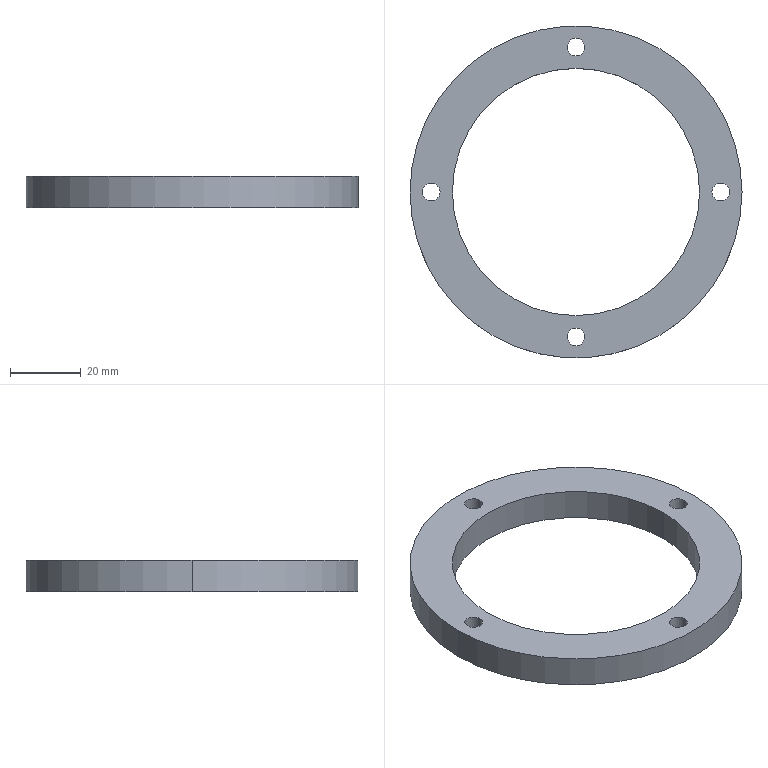Part | SolidWorks | features BaseBody 1 | 1 solid | 14 faces | box 94 x 94 x 9 mm | volume 27115 mm3 | cylinder 12 | plane 2 | commonest cylinder face diameters 5 x8 70 x2 94 x2
STEP:
#1=CARTESIAN_POINT('',(35.,0.,9.));
#2=VERTEX_POINT('',#1);
#3=CARTESIAN_POINT('',(-35.,0.,9.));
#4=VERTEX_POINT('',#3);
#5=CARTESIAN_POINT('',(0.,0.,9.));
#6=DIRECTION('',(0.,0.,-1.));
#7=DIRECTION('',(-1.,0.,0.));
#8=AXIS2_PLACEMENT_3D('',#5,#6,#7);
#9=CIRCLE('',#8,35.);
#10=EDGE_CURVE('',#2,#4,#9,.T.);
#11=ORIENTED_EDGE('',*,*,#10,.F.);
#12=CARTESIAN_POINT('',(35.,0.,0.));
#13=VERTEX_POINT('',#12);
#14=CARTESIAN_POINT('',(35.,0.,9.));
#15=DIRECTION('',(0.,0.,-1.));
#16=VECTOR('',#15,1000.);
#17=LINE('',#14,#16);
#18=EDGE_CURVE('',#2,#13,#17,.T.);
#19=ORIENTED_EDGE('',*,*,#18,.T.);
#20=CARTESIAN_POINT('',(-35.,0.,0.));
#21=VERTEX_POINT('',#20);
#22=CARTESIAN_POINT('',(0.,0.,0.));
#23=DIRECTION('',(0.,0.,1.));
#24=DIRECTION('',(-1.,0.,0.));
#25=AXIS2_PLACEMENT_3D('',#22,#23,#24);
#26=CIRCLE('',#25,35.);
#27=EDGE_CURVE('',#21,#13,#26,.T.);
#28=ORIENTED_EDGE('',*,*,#27,.F.);
#29=CARTESIAN_POINT('',(-35.,0.,9.));
#30=DIRECTION('',(0.,0.,-1.));
#31=VECTOR('',#30,1000.);
#32=LINE('',#29,#31);
#33=EDGE_CURVE('',#4,#21,#32,.T.);
#34=ORIENTED_EDGE('',*,*,#33,.F.);
#35=EDGE_LOOP('',(#11,#19,#28,#34));
#36=FACE_OUTER_BOUND('',#35,.T.);
#37=CARTESIAN_POINT('',(0.,0.,9.));
#38=DIRECTION('',(0.,0.,-1.));
#39=DIRECTION('',(-1.,0.,0.));
#40=AXIS2_PLACEMENT_3D('',#37,#38,#39);
#41=CYLINDRICAL_SURFACE('',#40,35.);
#42=ADVANCED_FACE('',(#36),#41,.F.);
#43=CARTESIAN_POINT('',(47.,0.,9.));
#44=VERTEX_POINT('',#43);
#45=CARTESIAN_POINT('',(-47.,0.,9.));
#46=VERTEX_POINT('',#45);
#47=CARTESIAN_POINT('',(0.,0.,9.));
#48=DIRECTION('',(0.,0.,1.));
#49=DIRECTION('',(-1.,0.,0.));
#50=AXIS2_PLACEMENT_3D('',#47,#48,#49);
#51=CIRCLE('',#50,47.);
#52=EDGE_CURVE('',#44,#46,#51,.T.);
#53=ORIENTED_EDGE('',*,*,#52,.F.);
#54=CARTESIAN_POINT('',(47.,0.,0.));
#55=VERTEX_POINT('',#54);
#56=CARTESIAN_POINT('',(47.,0.,9.));
#57=DIRECTION('',(0.,0.,-1.));
#58=VECTOR('',#57,1000.);
#59=LINE('',#56,#58);
#60=EDGE_CURVE('',#44,#55,#59,.T.);
#61=ORIENTED_EDGE('',*,*,#60,.T.);
#62=CARTESIAN_POINT('',(-47.,0.,0.));
#63=VERTEX_POINT('',#62);
#64=CARTESIAN_POINT('',(0.,0.,0.));
#65=DIRECTION('',(0.,0.,1.));
#66=DIRECTION('',(-1.,0.,0.));
#67=AXIS2_PLACEMENT_3D('',#64,#65,#66);
#68=CIRCLE('',#67,47.);
#69=EDGE_CURVE('',#55,#63,#68,.T.);
#70=ORIENTED_EDGE('',*,*,#69,.T.);
#71=CARTESIAN_POINT('',(-47.,0.,9.));
#72=DIRECTION('',(0.,0.,-1.));
#73=VECTOR('',#72,1000.);
#74=LINE('',#71,#73);
#75=EDGE_CURVE('',#46,#63,#74,.T.);
#76=ORIENTED_EDGE('',*,*,#75,.F.);
#77=EDGE_LOOP('',(#53,#61,#70,#76));
#78=FACE_OUTER_BOUND('',#77,.T.);
#79=CARTESIAN_POINT('',(0.,0.,9.));
#80=DIRECTION('',(0.,0.,-1.));
#81=DIRECTION('',(-1.,0.,0.));
#82=AXIS2_PLACEMENT_3D('',#79,#80,#81);
#83=CYLINDRICAL_SURFACE('',#82,47.);
#84=ADVANCED_FACE('',(#78),#83,.T.);
#85=CARTESIAN_POINT('',(-43.5,0.,0.));
#86=VERTEX_POINT('',#85);
#87=CARTESIAN_POINT('',(-38.5,0.,0.));
#88=VERTEX_POINT('',#87);
#89=CARTESIAN_POINT('',(-41.,0.,0.));
#90=DIRECTION('',(0.,0.,1.));
#91=DIRECTION('',(1.,0.,0.));
#92=AXIS2_PLACEMENT_3D('',#89,#90,#91);
#93=CIRCLE('',#92,2.5);
#94=EDGE_CURVE('',#86,#88,#93,.T.);
#95=ORIENTED_EDGE('',*,*,#94,.F.);
#96=CARTESIAN_POINT('',(-43.5,0.,9.));
#97=VERTEX_POINT('',#96);
#98=CARTESIAN_POINT('',(-43.5,0.,-34.));
#99=DIRECTION('',(0.,0.,1.));
#100=VECTOR('',#99,1000.);
#101=LINE('',#98,#100);
#102=EDGE_CURVE('',#86,#97,#101,.T.);
#103=ORIENTED_EDGE('',*,*,#102,.T.);
#104=CARTESIAN_POINT('',(-38.5,0.,9.));
#105=VERTEX_POINT('',#104);
#106=CARTESIAN_POINT('',(-41.,0.,9.));
#107=DIRECTION('',(0.,0.,-1.));
#108=DIRECTION('',(1.,0.,0.));
#109=AXIS2_PLACEMENT_3D('',#106,#107,#108);
#110=CIRCLE('',#109,2.5);
#111=EDGE_CURVE('',#105,#97,#110,.T.);
#112=ORIENTED_EDGE('',*,*,#111,.F.);
#113=CARTESIAN_POINT('',(-38.5,0.,-34.));
#114=DIRECTION('',(0.,0.,1.));
#115=VECTOR('',#114,1000.);
#116=LINE('',#113,#115);
#117=EDGE_CURVE('',#88,#105,#116,.T.);
#118=ORIENTED_EDGE('',*,*,#117,.F.);
#119=EDGE_LOOP('',(#95,#103,#112,#118));
#120=FACE_OUTER_BOUND('',#119,.T.);
#121=CARTESIAN_POINT('',(-41.,0.,-34.));
#122=DIRECTION('',(0.,0.,1.));
#123=DIRECTION('',(1.,0.,0.));
#124=AXIS2_PLACEMENT_3D('',#121,#122,#123);
#125=CYLINDRICAL_SURFACE('',#124,2.5);
#126=ADVANCED_FACE('',(#120),#125,.F.);
#127=CARTESIAN_POINT('',(-2.5,-41.,0.));
#128=VERTEX_POINT('',#127);
#129=CARTESIAN_POINT('',(2.5,-41.,0.));
#130=VERTEX_POINT('',#129);
#131=CARTESIAN_POINT('',(0.,-41.,0.));
#132=DIRECTION('',(0.,0.,1.));
#133=DIRECTION('',(1.,0.,0.));
#134=AXIS2_PLACEMENT_3D('',#131,#132,#133);
#135=CIRCLE('',#134,2.5);
#136=EDGE_CURVE('',#128,#130,#135,.T.);
#137=ORIENTED_EDGE('',*,*,#136,.F.);
#138=CARTESIAN_POINT('',(-2.5,-41.,9.));
#139=VERTEX_POINT('',#138);
#140=CARTESIAN_POINT('',(-2.5,-41.,-34.));
#141=DIRECTION('',(0.,0.,1.));
#142=VECTOR('',#141,1000.);
#143=LINE('',#140,#142);
#144=EDGE_CURVE('',#128,#139,#143,.T.);
#145=ORIENTED_EDGE('',*,*,#144,.T.);
#146=CARTESIAN_POINT('',(2.5,-41.,9.));
#147=VERTEX_POINT('',#146);
#148=CARTESIAN_POINT('',(0.,-41.,9.));
#149=DIRECTION('',(0.,0.,-1.));
#150=DIRECTION('',(1.,0.,0.));
#151=AXIS2_PLACEMENT_3D('',#148,#149,#150);
#152=CIRCLE('',#151,2.5);
#153=EDGE_CURVE('',#147,#139,#152,.T.);
#154=ORIENTED_EDGE('',*,*,#153,.F.);
#155=CARTESIAN_POINT('',(2.5,-41.,-34.));
#156=DIRECTION('',(0.,0.,1.));
#157=VECTOR('',#156,1000.);
#158=LINE('',#155,#157);
#159=EDGE_CURVE('',#130,#147,#158,.T.);
#160=ORIENTED_EDGE('',*,*,#159,.F.);
#161=EDGE_LOOP('',(#137,#145,#154,#160));
#162=FACE_OUTER_BOUND('',#161,.T.);
#163=CARTESIAN_POINT('',(0.,-41.,-34.));
#164=DIRECTION('',(0.,0.,1.));
#165=DIRECTION('',(1.,0.,0.));
#166=AXIS2_PLACEMENT_3D('',#163,#164,#165);
#167=CYLINDRICAL_SURFACE('',#166,2.5);
#168=ADVANCED_FACE('',(#162),#167,.F.);
#169=CARTESIAN_POINT('',(38.5,0.,0.));
#170=VERTEX_POINT('',#169);
#171=CARTESIAN_POINT('',(43.5,0.,0.));
#172=VERTEX_POINT('',#171);
#173=CARTESIAN_POINT('',(41.,0.,0.));
#174=DIRECTION('',(0.,0.,1.));
#175=DIRECTION('',(1.,0.,0.));
#176=AXIS2_PLACEMENT_3D('',#173,#174,#175);
#177=CIRCLE('',#176,2.5);
#178=EDGE_CURVE('',#170,#172,#177,.T.);
#179=ORIENTED_EDGE('',*,*,#178,.F.);
#180=CARTESIAN_POINT('',(38.5,0.,9.));
#181=VERTEX_POINT('',#180);
#182=CARTESIAN_POINT('',(38.5,0.,-34.));
#183=DIRECTION('',(0.,0.,1.));
#184=VECTOR('',#183,1000.);
#185=LINE('',#182,#184);
#186=EDGE_CURVE('',#170,#181,#185,.T.);
#187=ORIENTED_EDGE('',*,*,#186,.T.);
#188=CARTESIAN_POINT('',(43.5,0.,9.));
#189=VERTEX_POINT('',#188);
#190=CARTESIAN_POINT('',(41.,0.,9.));
#191=DIRECTION('',(0.,0.,-1.));
#192=DIRECTION('',(1.,0.,0.));
#193=AXIS2_PLACEMENT_3D('',#190,#191,#192);
#194=CIRCLE('',#193,2.5);
#195=EDGE_CURVE('',#189,#181,#194,.T.);
#196=ORIENTED_EDGE('',*,*,#195,.F.);
#197=CARTESIAN_POINT('',(43.5,0.,-34.));
#198=DIRECTION('',(0.,0.,1.));
#199=VECTOR('',#198,1000.);
#200=LINE('',#197,#199);
#201=EDGE_CURVE('',#172,#189,#200,.T.);
#202=ORIENTED_EDGE('',*,*,#201,.F.);
#203=EDGE_LOOP('',(#179,#187,#196,#202));
#204=FACE_OUTER_BOUND('',#203,.T.);
#205=CARTESIAN_POINT('',(41.,0.,-34.));
#206=DIRECTION('',(0.,0.,1.));
#207=DIRECTION('',(1.,0.,0.));
#208=AXIS2_PLACEMENT_3D('',#205,#206,#207);
#209=CYLINDRICAL_SURFACE('',#208,2.5);
#210=ADVANCED_FACE('',(#204),#209,.F.);
#211=CARTESIAN_POINT('',(-2.5,41.,0.));
#212=VERTEX_POINT('',#211);
#213=CARTESIAN_POINT('',(2.5,41.,0.));
#214=VERTEX_POINT('',#213);
#215=CARTESIAN_POINT('',(0.,41.,0.));
#216=DIRECTION('',(0.,0.,1.));
#217=DIRECTION('',(1.,0.,0.));
#218=AXIS2_PLACEMENT_3D('',#215,#216,#217);
#219=CIRCLE('',#218,2.5);
#220=EDGE_CURVE('',#212,#214,#219,.T.);
#221=ORIENTED_EDGE('',*,*,#220,.F.);
#222=CARTESIAN_POINT('',(-2.5,41.,9.));
#223=VERTEX_POINT('',#222);
#224=CARTESIAN_POINT('',(-2.5,41.,-34.));
#225=DIRECTION('',(0.,0.,1.));
#226=VECTOR('',#225,1000.);
#227=LINE('',#224,#226);
#228=EDGE_CURVE('',#212,#223,#227,.T.);
#229=ORIENTED_EDGE('',*,*,#228,.T.);
#230=CARTESIAN_POINT('',(2.5,41.,9.));
#231=VERTEX_POINT('',#230);
#232=CARTESIAN_POINT('',(0.,41.,9.));
#233=DIRECTION('',(0.,0.,-1.));
#234=DIRECTION('',(1.,0.,0.));
#235=AXIS2_PLACEMENT_3D('',#232,#233,#234);
#236=CIRCLE('',#235,2.5);
#237=EDGE_CURVE('',#231,#223,#236,.T.);
#238=ORIENTED_EDGE('',*,*,#237,.F.);
#239=CARTESIAN_POINT('',(2.5,41.,-34.));
#240=DIRECTION('',(0.,0.,1.));
#241=VECTOR('',#240,1000.);
#242=LINE('',#239,#241);
#243=EDGE_CURVE('',#214,#231,#242,.T.);
#244=ORIENTED_EDGE('',*,*,#243,.F.);
#245=EDGE_LOOP('',(#221,#229,#238,#244));
#246=FACE_OUTER_BOUND('',#245,.T.);
#247=CARTESIAN_POINT('',(0.,41.,-34.));
#248=DIRECTION('',(0.,0.,1.));
#249=DIRECTION('',(1.,0.,0.));
#250=AXIS2_PLACEMENT_3D('',#247,#248,#249);
#251=CYLINDRICAL_SURFACE('',#250,2.5);
#252=ADVANCED_FACE('',(#246),#251,.F.);
#253=CARTESIAN_POINT('',(0.,0.,9.));
#254=DIRECTION('',(0.,0.,-1.));
#255=DIRECTION('',(-1.,0.,0.));
#256=AXIS2_PLACEMENT_3D('',#253,#254,#255);
#257=CIRCLE('',#256,35.);
#258=EDGE_CURVE('',#4,#2,#257,.T.);
#259=ORIENTED_EDGE('',*,*,#258,.T.);
#260=ORIENTED_EDGE('',*,*,#10,.T.);
#261=EDGE_LOOP('',(#259,#260));
#262=FACE_BOUND('',#261,.T.);
#263=CARTESIAN_POINT('',(0.,0.,9.));
#264=DIRECTION('',(0.,0.,1.));
#265=DIRECTION('',(-1.,0.,0.));
#266=AXIS2_PLACEMENT_3D('',#263,#264,#265);
#267=CIRCLE('',#266,47.);
#268=EDGE_CURVE('',#46,#44,#267,.T.);
#269=ORIENTED_EDGE('',*,*,#268,.T.);
#270=ORIENTED_EDGE('',*,*,#52,.T.);
#271=EDGE_LOOP('',(#269,#270));
#272=FACE_OUTER_BOUND('',#271,.T.);
#273=ORIENTED_EDGE('',*,*,#111,.T.);
#274=CARTESIAN_POINT('',(-41.,0.,9.));
#275=DIRECTION('',(0.,0.,-1.));
#276=DIRECTION('',(1.,0.,0.));
#277=AXIS2_PLACEMENT_3D('',#274,#275,#276);
#278=CIRCLE('',#277,2.5);
#279=EDGE_CURVE('',#97,#105,#278,.T.);
#280=ORIENTED_EDGE('',*,*,#279,.T.);
#281=EDGE_LOOP('',(#273,#280));
#282=FACE_BOUND('',#281,.T.);
#283=ORIENTED_EDGE('',*,*,#153,.T.);
#284=CARTESIAN_POINT('',(0.,-41.,9.));
#285=DIRECTION('',(0.,0.,-1.));
#286=DIRECTION('',(1.,0.,0.));
#287=AXIS2_PLACEMENT_3D('',#284,#285,#286);
#288=CIRCLE('',#287,2.5);
#289=EDGE_CURVE('',#139,#147,#288,.T.);
#290=ORIENTED_EDGE('',*,*,#289,.T.);
#291=EDGE_LOOP('',(#283,#290));
#292=FACE_BOUND('',#291,.T.);
#293=ORIENTED_EDGE('',*,*,#195,.T.);
#294=CARTESIAN_POINT('',(41.,0.,9.));
#295=DIRECTION('',(0.,0.,-1.));
#296=DIRECTION('',(1.,0.,0.));
#297=AXIS2_PLACEMENT_3D('',#294,#295,#296);
#298=CIRCLE('',#297,2.5);
#299=EDGE_CURVE('',#181,#189,#298,.T.);
#300=ORIENTED_EDGE('',*,*,#299,.T.);
#301=EDGE_LOOP('',(#293,#300));
#302=FACE_BOUND('',#301,.T.);
#303=ORIENTED_EDGE('',*,*,#237,.T.);
#304=CARTESIAN_POINT('',(0.,41.,9.));
#305=DIRECTION('',(0.,0.,-1.));
#306=DIRECTION('',(1.,0.,0.));
#307=AXIS2_PLACEMENT_3D('',#304,#305,#306);
#308=CIRCLE('',#307,2.5);
#309=EDGE_CURVE('',#223,#231,#308,.T.);
#310=ORIENTED_EDGE('',*,*,#309,.T.);
#311=EDGE_LOOP('',(#303,#310));
#312=FACE_BOUND('',#311,.T.);
#313=CARTESIAN_POINT('',(0.,0.,9.));
#314=DIRECTION('',(0.,0.,1.));
#315=DIRECTION('',(1.,0.,0.));
#316=AXIS2_PLACEMENT_3D('',#313,#314,#315);
#317=PLANE('',#316);
#318=ADVANCED_FACE('',(#262,#272,#282,#292,#302,#312),#317,.T.);
#319=ORIENTED_EDGE('',*,*,#18,.F.);
#320=ORIENTED_EDGE('',*,*,#258,.F.);
#321=ORIENTED_EDGE('',*,*,#33,.T.);
#322=CARTESIAN_POINT('',(0.,0.,0.));
#323=DIRECTION('',(0.,0.,1.));
#324=DIRECTION('',(-1.,0.,0.));
#325=AXIS2_PLACEMENT_3D('',#322,#323,#324);
#326=CIRCLE('',#325,35.);
#327=EDGE_CURVE('',#13,#21,#326,.T.);
#328=ORIENTED_EDGE('',*,*,#327,.F.);
#329=EDGE_LOOP('',(#319,#320,#321,#328));
#330=FACE_OUTER_BOUND('',#329,.T.);
#331=CARTESIAN_POINT('',(0.,0.,9.));
#332=DIRECTION('',(0.,0.,-1.));
#333=DIRECTION('',(-1.,0.,0.));
#334=AXIS2_PLACEMENT_3D('',#331,#332,#333);
#335=CYLINDRICAL_SURFACE('',#334,35.);
#336=ADVANCED_FACE('',(#330),#335,.F.);
#337=ORIENTED_EDGE('',*,*,#60,.F.);
#338=ORIENTED_EDGE('',*,*,#268,.F.);
#339=ORIENTED_EDGE('',*,*,#75,.T.);
#340=CARTESIAN_POINT('',(0.,0.,0.));
#341=DIRECTION('',(0.,0.,1.));
#342=DIRECTION('',(-1.,0.,0.));
#343=AXIS2_PLACEMENT_3D('',#340,#341,#342);
#344=CIRCLE('',#343,47.);
#345=EDGE_CURVE('',#63,#55,#344,.T.);
#346=ORIENTED_EDGE('',*,*,#345,.T.);
#347=EDGE_LOOP('',(#337,#338,#339,#346));
#348=FACE_OUTER_BOUND('',#347,.T.);
#349=CARTESIAN_POINT('',(0.,0.,9.));
#350=DIRECTION('',(0.,0.,-1.));
#351=DIRECTION('',(-1.,0.,0.));
#352=AXIS2_PLACEMENT_3D('',#349,#350,#351);
#353=CYLINDRICAL_SURFACE('',#352,47.);
#354=ADVANCED_FACE('',(#348),#353,.T.);
#355=ORIENTED_EDGE('',*,*,#102,.F.);
#356=CARTESIAN_POINT('',(-41.,0.,0.));
#357=DIRECTION('',(0.,0.,1.));
#358=DIRECTION('',(1.,0.,0.));
#359=AXIS2_PLACEMENT_3D('',#356,#357,#358);
#360=CIRCLE('',#359,2.5);
#361=EDGE_CURVE('',#88,#86,#360,.T.);
#362=ORIENTED_EDGE('',*,*,#361,.F.);
#363=ORIENTED_EDGE('',*,*,#117,.T.);
#364=ORIENTED_EDGE('',*,*,#279,.F.);
#365=EDGE_LOOP('',(#355,#362,#363,#364));
#366=FACE_OUTER_BOUND('',#365,.T.);
#367=CARTESIAN_POINT('',(-41.,0.,-34.));
#368=DIRECTION('',(0.,0.,1.));
#369=DIRECTION('',(1.,0.,0.));
#370=AXIS2_PLACEMENT_3D('',#367,#368,#369);
#371=CYLINDRICAL_SURFACE('',#370,2.5);
#372=ADVANCED_FACE('',(#366),#371,.F.);
#373=ORIENTED_EDGE('',*,*,#144,.F.);
#374=CARTESIAN_POINT('',(0.,-41.,0.));
#375=DIRECTION('',(0.,0.,1.));
#376=DIRECTION('',(1.,0.,0.));
#377=AXIS2_PLACEMENT_3D('',#374,#375,#376);
#378=CIRCLE('',#377,2.5);
#379=EDGE_CURVE('',#130,#128,#378,.T.);
#380=ORIENTED_EDGE('',*,*,#379,.F.);
#381=ORIENTED_EDGE('',*,*,#159,.T.);
#382=ORIENTED_EDGE('',*,*,#289,.F.);
#383=EDGE_LOOP('',(#373,#380,#381,#382));
#384=FACE_OUTER_BOUND('',#383,.T.);
#385=CARTESIAN_POINT('',(0.,-41.,-34.));
#386=DIRECTION('',(0.,0.,1.));
#387=DIRECTION('',(1.,0.,0.));
#388=AXIS2_PLACEMENT_3D('',#385,#386,#387);
#389=CYLINDRICAL_SURFACE('',#388,2.5);
#390=ADVANCED_FACE('',(#384),#389,.F.);
#391=ORIENTED_EDGE('',*,*,#186,.F.);
#392=CARTESIAN_POINT('',(41.,0.,0.));
#393=DIRECTION('',(0.,0.,1.));
#394=DIRECTION('',(1.,0.,0.));
#395=AXIS2_PLACEMENT_3D('',#392,#393,#394);
#396=CIRCLE('',#395,2.5);
#397=EDGE_CURVE('',#172,#170,#396,.T.);
#398=ORIENTED_EDGE('',*,*,#397,.F.);
#399=ORIENTED_EDGE('',*,*,#201,.T.);
#400=ORIENTED_EDGE('',*,*,#299,.F.);
#401=EDGE_LOOP('',(#391,#398,#399,#400));
#402=FACE_OUTER_BOUND('',#401,.T.);
#403=CARTESIAN_POINT('',(41.,0.,-34.));
#404=DIRECTION('',(0.,0.,1.));
#405=DIRECTION('',(1.,0.,0.));
#406=AXIS2_PLACEMENT_3D('',#403,#404,#405);
#407=CYLINDRICAL_SURFACE('',#406,2.5);
#408=ADVANCED_FACE('',(#402),#407,.F.);
#409=ORIENTED_EDGE('',*,*,#228,.F.);
#410=CARTESIAN_POINT('',(0.,41.,0.));
#411=DIRECTION('',(0.,0.,1.));
#412=DIRECTION('',(1.,0.,0.));
#413=AXIS2_PLACEMENT_3D('',#410,#411,#412);
#414=CIRCLE('',#413,2.5);
#415=EDGE_CURVE('',#214,#212,#414,.T.);
#416=ORIENTED_EDGE('',*,*,#415,.F.);
#417=ORIENTED_EDGE('',*,*,#243,.T.);
#418=ORIENTED_EDGE('',*,*,#309,.F.);
#419=EDGE_LOOP('',(#409,#416,#417,#418));
#420=FACE_OUTER_BOUND('',#419,.T.);
#421=CARTESIAN_POINT('',(0.,41.,-34.));
#422=DIRECTION('',(0.,0.,1.));
#423=DIRECTION('',(1.,0.,0.));
#424=AXIS2_PLACEMENT_3D('',#421,#422,#423);
#425=CYLINDRICAL_SURFACE('',#424,2.5);
#426=ADVANCED_FACE('',(#420),#425,.F.);
#427=ORIENTED_EDGE('',*,*,#27,.T.);
#428=ORIENTED_EDGE('',*,*,#327,.T.);
#429=EDGE_LOOP('',(#427,#428));
#430=FACE_BOUND('',#429,.T.);
#431=ORIENTED_EDGE('',*,*,#345,.F.);
#432=ORIENTED_EDGE('',*,*,#69,.F.);
#433=EDGE_LOOP('',(#431,#432));
#434=FACE_OUTER_BOUND('',#433,.T.);
#435=ORIENTED_EDGE('',*,*,#361,.T.);
#436=ORIENTED_EDGE('',*,*,#94,.T.);
#437=EDGE_LOOP('',(#435,#436));
#438=FACE_BOUND('',#437,.T.);
#439=ORIENTED_EDGE('',*,*,#379,.T.);
#440=ORIENTED_EDGE('',*,*,#136,.T.);
#441=EDGE_LOOP('',(#439,#440));
#442=FACE_BOUND('',#441,.T.);
#443=ORIENTED_EDGE('',*,*,#397,.T.);
#444=ORIENTED_EDGE('',*,*,#178,.T.);
#445=EDGE_LOOP('',(#443,#444));
#446=FACE_BOUND('',#445,.T.);
#447=ORIENTED_EDGE('',*,*,#415,.T.);
#448=ORIENTED_EDGE('',*,*,#220,.T.);
#449=EDGE_LOOP('',(#447,#448));
#450=FACE_BOUND('',#449,.T.);
#451=CARTESIAN_POINT('',(0.,0.,0.));
#452=DIRECTION('',(0.,0.,1.));
#453=DIRECTION('',(1.,0.,0.));
#454=AXIS2_PLACEMENT_3D('',#451,#452,#453);
#455=PLANE('',#454);
#456=ADVANCED_FACE('',(#430,#434,#438,#442,#446,#450),#455,.F.);
#457=CLOSED_SHELL('',(#42,#84,#126,#168,#210,#252,#318,#336,#354,#372,#390,#408,#426,#456));
#458=MANIFOLD_SOLID_BREP('',#457);
#459=CARTESIAN_POINT('',(0.,0.,0.));
#460=DIRECTION('',(0.,0.,1.));
#461=DIRECTION('',(1.,0.,0.));
#462=AXIS2_PLACEMENT_3D('',#459,#460,#461);
#463=(LENGTH_UNIT()NAMED_UNIT(*)SI_UNIT(.MILLI.,.METRE.));
#464=UNCERTAINTY_MEASURE_WITH_UNIT(LENGTH_MEASURE(0.00001),#463,'','');
#465=(NAMED_UNIT(*)PLANE_ANGLE_UNIT()SI_UNIT($,.RADIAN.));
#466=(NAMED_UNIT(*)SI_UNIT($,.STERADIAN.)SOLID_ANGLE_UNIT());
#467=(GEOMETRIC_REPRESENTATION_CONTEXT(3)GLOBAL_UNCERTAINTY_ASSIGNED_CONTEXT((#464))GLOBAL_UNIT_ASSIGNED_CONTEXT((#463,#465,#466))REPRESENTATION_CONTEXT('',''));
#468=ADVANCED_BREP_SHAPE_REPRESENTATION('',(#458,#462),#467);